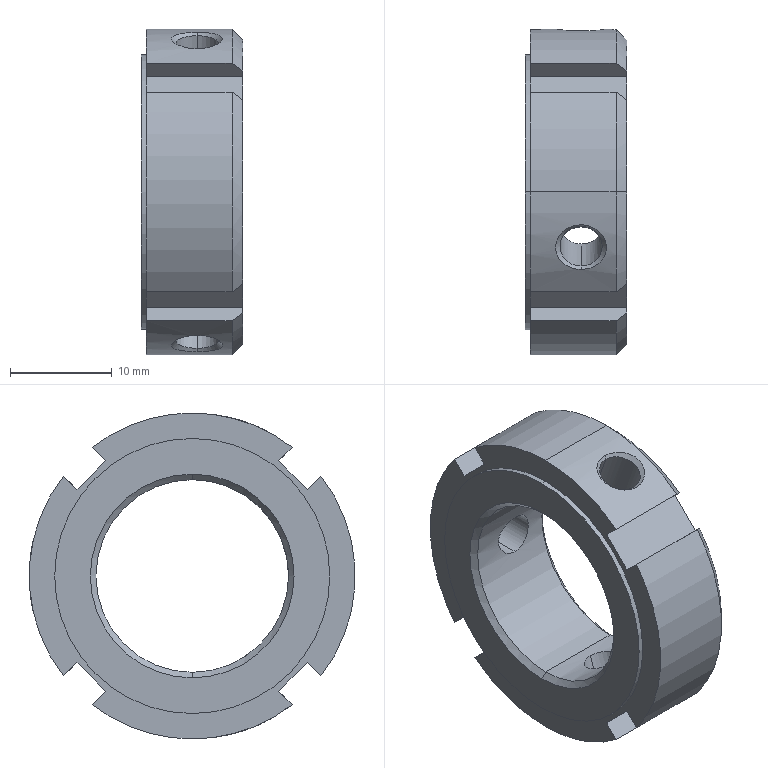Part | STEP file | _PLNY20x | 1 solid | 50 faces | box 10 x 32 x 32 mm | volume 4486 mm3 | plane 16 | cone 16 | cylinder 16 | torus 2 | commonest cylinder face diameters 4.134 x6 32 x6 18.917 x2 27 x2